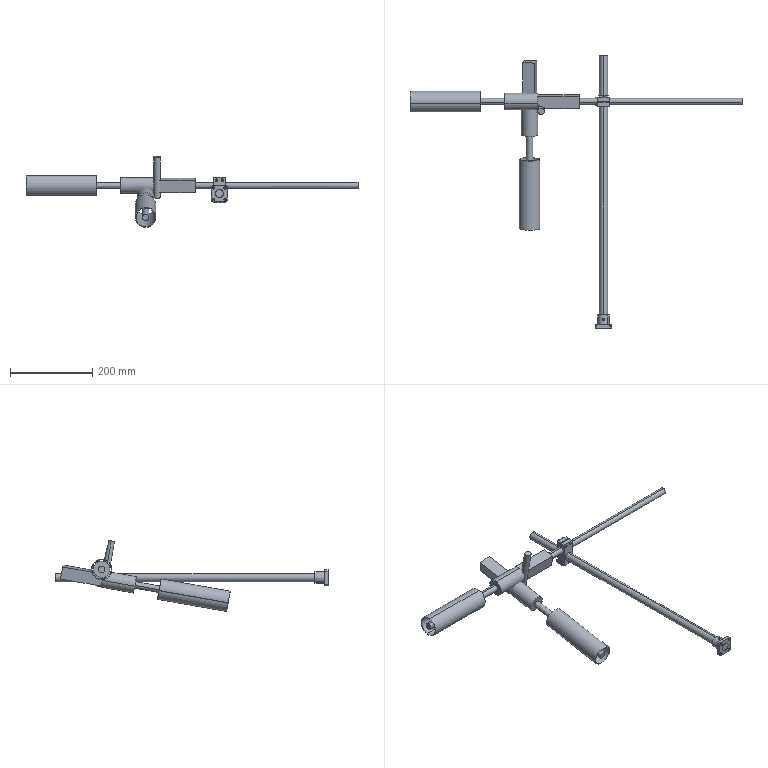Part | SolidWorks | features AEMSimFeature 1 | 13 solids | 198 faces | box 805 x 660 x 172.187 mm | volume 944058 mm3 | plane 106 | cylinder 80 | torus 8 | cone 4 | commonest cylinder face diameters 50 x9 4.918 x8 5.5 x8 6 x8 6.6 x8 9.6 x8